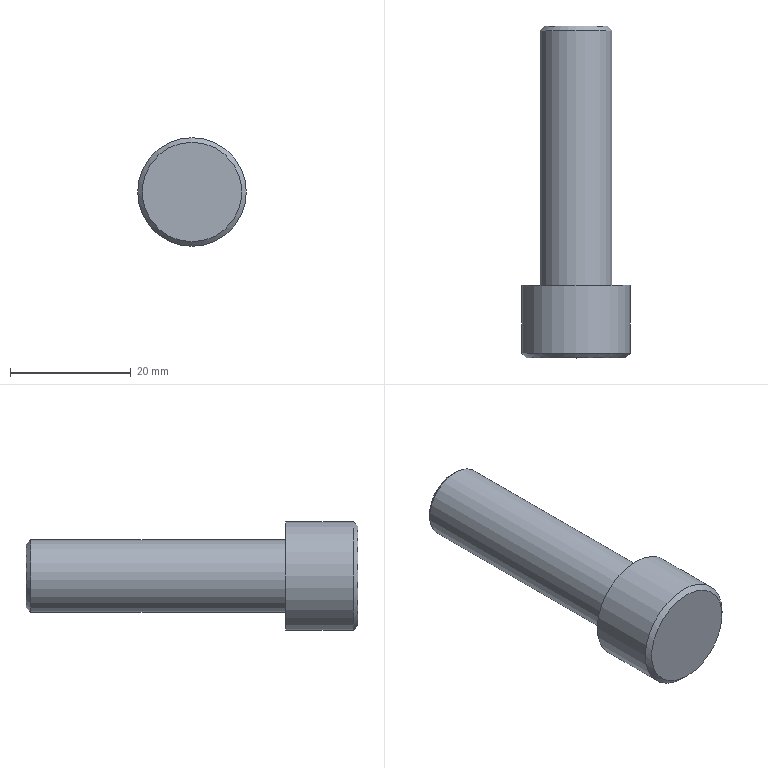Part | STEP file | SCREW-2_id366_x_t | 1 solid | 7 faces | box 18 x 55 x 18 mm | volume 7891 mm3 | plane 3 | cone 2 | cylinder 2 | commonest cylinder face diameters 12 x1 18 x1
STEP:
#1=CARTESIAN_POINT('',(-165.,-289.5,129.25));
#2=VERTEX_POINT('',#1);
#3=CARTESIAN_POINT('',(-165.,-289.5,121.));
#4=DIRECTION('',(0.,1.,0.));
#5=DIRECTION('',(0.,0.,1.));
#6=AXIS2_PLACEMENT_3D('',#3,#4,#5);
#7=CIRCLE('',#6,8.25);
#8=EDGE_CURVE('',#2,#2,#7,.T.);
#9=ORIENTED_EDGE('',*,*,#8,.F.);
#10=EDGE_LOOP('',(#9));
#11=FACE_OUTER_BOUND('',#10,.T.);
#12=CARTESIAN_POINT('',(-165.,-289.5,121.));
#13=DIRECTION('',(0.,-1.,0.));
#14=DIRECTION('',(0.,0.,-1.));
#15=AXIS2_PLACEMENT_3D('',#12,#13,#14);
#16=PLANE('',#15);
#17=ADVANCED_FACE('',(#11),#16,.T.);
#18=ORIENTED_EDGE('',*,*,#8,.T.);
#19=EDGE_LOOP('',(#18));
#20=FACE_BOUND('',#19,.T.);
#21=CARTESIAN_POINT('',(-165.,-288.75,112.));
#22=VERTEX_POINT('',#21);
#23=CARTESIAN_POINT('',(-165.,-288.75,121.));
#24=DIRECTION('',(0.,1.,0.));
#25=DIRECTION('',(0.,0.,-1.));
#26=AXIS2_PLACEMENT_3D('',#23,#24,#25);
#27=CIRCLE('',#26,9.);
#28=EDGE_CURVE('',#22,#22,#27,.T.);
#29=ORIENTED_EDGE('',*,*,#28,.F.);
#30=EDGE_LOOP('',(#29));
#31=FACE_BOUND('',#30,.T.);
#32=CARTESIAN_POINT('',(-165.,-288.75,121.));
#33=DIRECTION('',(0.,1.,0.));
#34=DIRECTION('',(0.,0.,1.));
#35=AXIS2_PLACEMENT_3D('',#32,#33,#34);
#36=CONICAL_SURFACE('',#35,9.,45.);
#37=ADVANCED_FACE('',(#20,#31),#36,.T.);
#38=CARTESIAN_POINT('',(-165.,-234.5,115.75));
#39=VERTEX_POINT('',#38);
#40=CARTESIAN_POINT('',(-165.,-234.5,121.));
#41=DIRECTION('',(0.,-1.,0.));
#42=DIRECTION('',(0.,0.,-1.));
#43=AXIS2_PLACEMENT_3D('',#40,#41,#42);
#44=CIRCLE('',#43,5.25);
#45=EDGE_CURVE('',#39,#39,#44,.T.);
#46=ORIENTED_EDGE('',*,*,#45,.F.);
#47=EDGE_LOOP('',(#46));
#48=FACE_OUTER_BOUND('',#47,.T.);
#49=CARTESIAN_POINT('',(-165.,-234.5,121.));
#50=DIRECTION('',(0.,-1.,0.));
#51=DIRECTION('',(0.,0.,-1.));
#52=AXIS2_PLACEMENT_3D('',#49,#50,#51);
#53=PLANE('',#52);
#54=ADVANCED_FACE('',(#48),#53,.F.);
#55=ORIENTED_EDGE('',*,*,#28,.T.);
#56=EDGE_LOOP('',(#55));
#57=FACE_BOUND('',#56,.T.);
#58=CARTESIAN_POINT('',(-165.,-277.5,112.));
#59=VERTEX_POINT('',#58);
#60=CARTESIAN_POINT('',(-165.,-277.5,121.));
#61=DIRECTION('',(0.,-1.,0.));
#62=DIRECTION('',(0.,0.,-1.));
#63=AXIS2_PLACEMENT_3D('',#60,#61,#62);
#64=CIRCLE('',#63,9.);
#65=EDGE_CURVE('',#59,#59,#64,.T.);
#66=ORIENTED_EDGE('',*,*,#65,.T.);
#67=EDGE_LOOP('',(#66));
#68=FACE_BOUND('',#67,.T.);
#69=CARTESIAN_POINT('',(-165.,-292.25,121.));
#70=DIRECTION('',(0.,-1.,0.));
#71=DIRECTION('',(0.,0.,-1.));
#72=AXIS2_PLACEMENT_3D('',#69,#70,#71);
#73=CYLINDRICAL_SURFACE('',#72,9.);
#74=ADVANCED_FACE('',(#57,#68),#73,.T.);
#75=CARTESIAN_POINT('',(-165.,-235.25,115.));
#76=VERTEX_POINT('',#75);
#77=CARTESIAN_POINT('',(-165.,-235.25,121.));
#78=DIRECTION('',(0.,-1.,0.));
#79=DIRECTION('',(0.,0.,-1.));
#80=AXIS2_PLACEMENT_3D('',#77,#78,#79);
#81=CIRCLE('',#80,6.);
#82=EDGE_CURVE('',#76,#76,#81,.T.);
#83=ORIENTED_EDGE('',*,*,#82,.F.);
#84=EDGE_LOOP('',(#83));
#85=FACE_BOUND('',#84,.T.);
#86=ORIENTED_EDGE('',*,*,#45,.T.);
#87=EDGE_LOOP('',(#86));
#88=FACE_BOUND('',#87,.T.);
#89=CARTESIAN_POINT('',(-165.,-235.25,121.));
#90=DIRECTION('',(0.,-1.,0.));
#91=DIRECTION('',(0.,0.,-1.));
#92=AXIS2_PLACEMENT_3D('',#89,#90,#91);
#93=CONICAL_SURFACE('',#92,6.,45.);
#94=ADVANCED_FACE('',(#85,#88),#93,.T.);
#95=CARTESIAN_POINT('',(-165.,-277.5,115.));
#96=VERTEX_POINT('',#95);
#97=CARTESIAN_POINT('',(-165.,-277.5,121.));
#98=DIRECTION('',(0.,1.,0.));
#99=DIRECTION('',(0.,0.,-1.));
#100=AXIS2_PLACEMENT_3D('',#97,#98,#99);
#101=CIRCLE('',#100,6.);
#102=EDGE_CURVE('',#96,#96,#101,.T.);
#103=ORIENTED_EDGE('',*,*,#102,.F.);
#104=EDGE_LOOP('',(#103));
#105=FACE_BOUND('',#104,.T.);
#106=ORIENTED_EDGE('',*,*,#65,.F.);
#107=EDGE_LOOP('',(#106));
#108=FACE_BOUND('',#107,.T.);
#109=CARTESIAN_POINT('',(-165.,-277.5,121.));
#110=DIRECTION('',(0.,-1.,0.));
#111=DIRECTION('',(0.,0.,-1.));
#112=AXIS2_PLACEMENT_3D('',#109,#110,#111);
#113=PLANE('',#112);
#114=ADVANCED_FACE('',(#105,#108),#113,.F.);
#115=ORIENTED_EDGE('',*,*,#102,.T.);
#116=EDGE_LOOP('',(#115));
#117=FACE_BOUND('',#116,.T.);
#118=ORIENTED_EDGE('',*,*,#82,.T.);
#119=EDGE_LOOP('',(#118));
#120=FACE_BOUND('',#119,.T.);
#121=CARTESIAN_POINT('',(-165.,-292.25,121.));
#122=DIRECTION('',(0.,-1.,0.));
#123=DIRECTION('',(0.,0.,-1.));
#124=AXIS2_PLACEMENT_3D('',#121,#122,#123);
#125=CYLINDRICAL_SURFACE('',#124,6.);
#126=ADVANCED_FACE('',(#117,#120),#125,.T.);
#127=CLOSED_SHELL('',(#17,#37,#54,#74,#94,#114,#126));
#128=MANIFOLD_SOLID_BREP('',#127);
#129=(LENGTH_UNIT()NAMED_UNIT(*)SI_UNIT(.MILLI.,.METRE.));
#130=UNCERTAINTY_MEASURE_WITH_UNIT(LENGTH_MEASURE(0.00002),#129,'','');
#131=(NAMED_UNIT(*)PLANE_ANGLE_UNIT()SI_UNIT($,.RADIAN.));
#132=PLANE_ANGLE_MEASURE_WITH_UNIT(PLANE_ANGLE_MEASURE(0.01745),#131);
#133=DIMENSIONAL_EXPONENTS(0.,0.,0.,0.,0.,0.,0.);
#134=(CONVERSION_BASED_UNIT('DEGREE',#132)NAMED_UNIT(#133)PLANE_ANGLE_UNIT());
#135=(NAMED_UNIT(*)SI_UNIT($,.STERADIAN.)SOLID_ANGLE_UNIT());
#136=(GEOMETRIC_REPRESENTATION_CONTEXT(3)GLOBAL_UNCERTAINTY_ASSIGNED_CONTEXT((#130))GLOBAL_UNIT_ASSIGNED_CONTEXT((#129,#134,#135))REPRESENTATION_CONTEXT('',''));
#137=ADVANCED_BREP_SHAPE_REPRESENTATION('',(#128),#136);